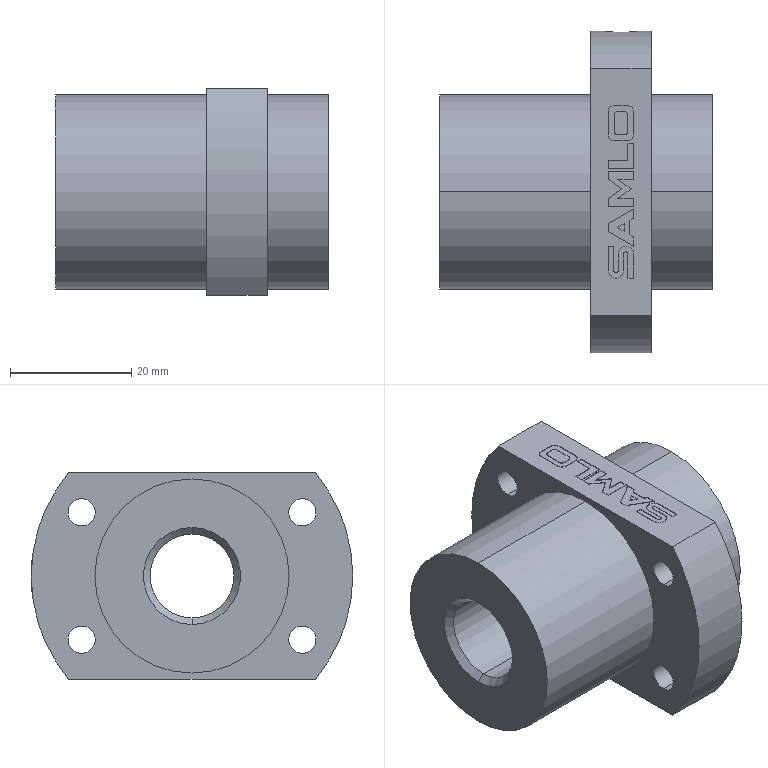Part | SolidWorks | features BaseBody 1 | 1 solid | 94 faces | box 45 x 53 x 34 mm | volume 37006 mm3 | plane 58 | cylinder 30 | cone 6 | commonest cylinder face diameters 4.5 x8 0.965 x4 2.045 x4 32 x4 0.691 x2 2.535 x2